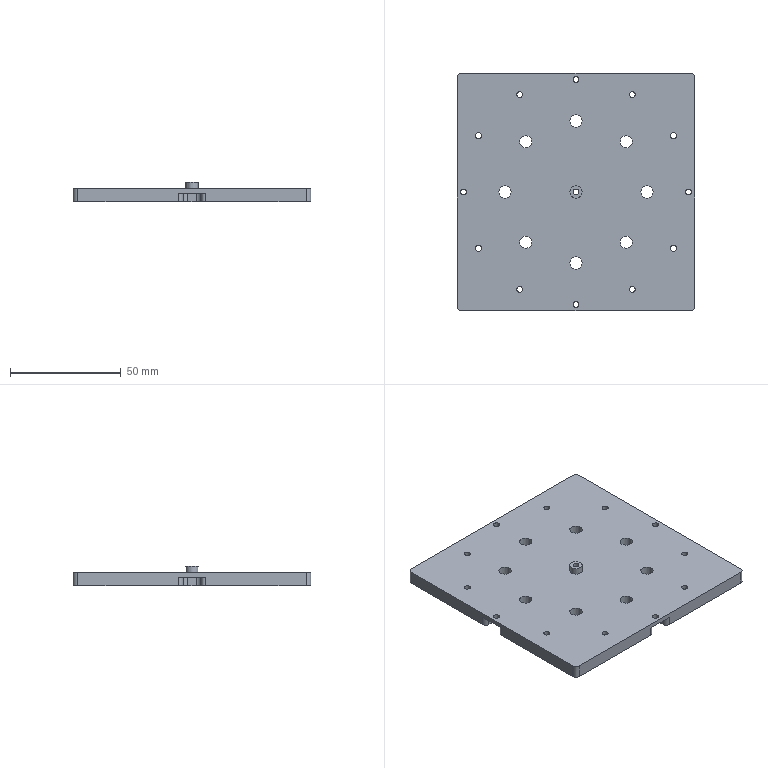Part | STEP file | Combiner cover | 1 solid | 179 faces | box 107 x 107 x 9 mm | volume 64733 mm3 | cylinder 83 | cone 64 | plane 32 | commonest cylinder face diameters 2.05 x32 4 x20 2.7 x13 5.5 x9 7 x9